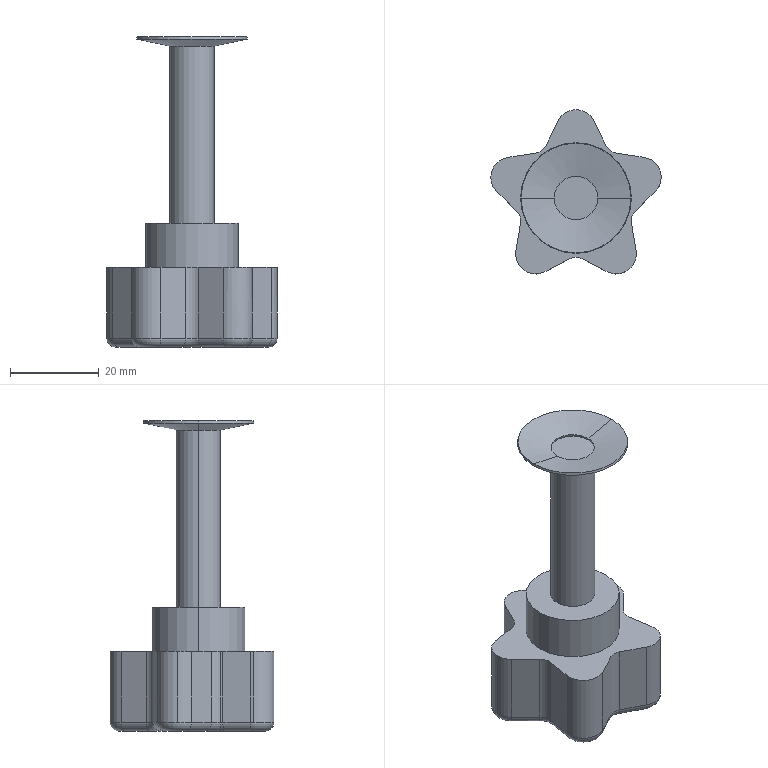Part | STEP file | Five-star handle (with gland) 2 (M10_40_40) | 2 solids | 62 faces | box 38.486 x 37.046 x 70.083 mm | volume 22563 mm3 | cylinder 27 | plane 14 | torus 13 | cone 8 | commonest cylinder face diameters 4 x10 9.069 x7 6 x6 10 x2 21 x2